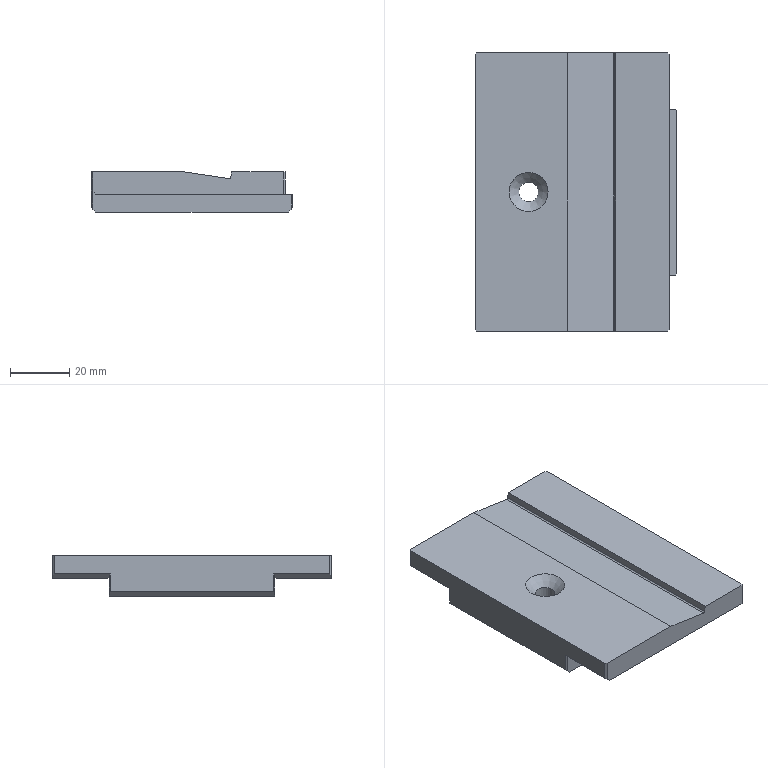NC program | NX | posted with a generic post | part box 68 x 94 x 13.65 mm
Lines 1 to 1097 of 5620:
N10 G17 G21 G94 G90
(一刀光面 , TOOL : D50面刀)
N12 T01 M6
N14 G54
N16 G17 G0 G90 X78.5 Y-22.5 B0. C0. S3500 M3
N18 G43 Z30. H1
N20 Z3.
N22 G94 G1 Z0. F800.
N24 X73.5
N26 X-73.5
N28 X-78.5
N30 Z3.
N32 G0 Z30.
N34 X78.5 Y15.
N36 Z3.
N38 G1 Z0.
N40 X73.5
N42 X-73.5
N44 X-78.5
N46 Z3.
N48 G0 Z30.
N50 M5
(ADAPTIVE_MILLING , TOOL : D12开粗)
N52 T02 M6
N54 G54
N56 G17 G0 G90 X0.814 Y-47.076 B0. C0. S6500 M3
N58 G43 Z30. H2
N60 Z-13.
N62 G94 G1 Y-46.926 Z-13.937 F2500.
N64 Y-46.776 Z-14.308
N66 Y-46.626 Z-14.58
N68 X0.815 Y-46.476 Z-14.8
N70 Y-46.326 Z-14.984
N72 Y-46.176 Z-15.142
N74 X0.816 Y-46.026 Z-15.28
N76 Y-45.876 Z-15.4
N78 Y-45.726 Z-15.505
N80 X0.817 Y-45.576 Z-15.598
N82 Y-45.426 Z-15.679
N84 Y-45.276 Z-15.75
N86 X0.818 Y-45.126 Z-15.81
N88 Y-44.976 Z-15.862
N90 Y-44.826 Z-15.905
N92 X0.819 Y-44.676 Z-15.939
N94 Y-44.526 Z-15.966
N96 Y-44.376 Z-15.985
N98 X0.82 Y-44.226 Z-15.996
N100 Y-44.076 Z-16.
N102 X0.824 Y-42.206
N104 G3 X0.012 Y-41.059 R1.212
N106 X-2.89 Y-40.578 R11.249
N108 X-11.498 Y-40.406 R147.652
N110 G1 X-18.236 Y-40.4
N112 X-45.986 Y-40.399
N114 G2 X-48.611 Y-39.755 R6.142
N116 G1 X-48.855 Y-39.681
N118 X-49.918 Y-39.113
N120 G2 X-52.114 Y-36.915 R10.677
N122 X-52.788 Y-35.571 R9.839
N124 X-53.72 Y-30.116 R21.533
N126 X-53.893 Y-21.344 R159.693
N128 G1 X-53.899 Y-14.594
N130 X-53.898 Y32.484
N132 G2 X-51.638 Y37.222 R6.591
N134 X-46.864 Y39.623 R10.72
N136 X-40.988 Y40.3 R29.653
N138 X-27.714 Y40.399 R443.721
N140 G1 X46.082 Y40.397
N142 G2 X50.795 Y38.079 R6.624
N144 X53.148 Y33.282 R10.797
N146 X53.803 Y27.403 R30.317
N148 X53.899 Y13.453 R504.778
N150 G1 X53.898 Y-32.465
N152 G2 X52.294 Y-36.579 R6.493
N154 G1 X52.113 Y-36.918
N156 G2 X49.915 Y-39.114 R10.677
N158 G1 X48.852 Y-39.682
N160 X47.551 Y-40.06
N162 G2 X39.986 Y-40.38 R73.937
N164 G1 X30.536 Y-40.399
N166 X-42.041 Y-40.394
N168 G3 X-43.223 Y-40.15 R35.364
N170 G1 X-46.501
N172 X-47.701 Y-40.031
N174 X-48.855 Y-39.681
N176 X-49.918 Y-39.113
N178 G2 X-52.114 Y-36.915 R10.677
N180 G1 X-52.682 Y-35.852
N182 X-53.032 Y-34.698
N184 X-53.15 Y-33.499
N186 G3 X-53.259 Y-25.386 R401.161
N188 G1 X-53.298 Y-13.836
N190 Y29.859
N192 G2 X-52.591 Y33.461 R9.973
N194 X-48.087 Y37.818 R9.638
N196 X-42.325 Y39.395 R17.668
N198 X-34.538 Y39.77 R72.985
N200 G1 X-29.459 Y39.811
N202 X-28.698 Y40.032
N204 X-27.499 Y40.15
N206 X27.501
N208 G3 X34.729 Y39.821 R67.085
N210 G1 X43.91 Y39.783
N212 G2 X50.284 Y36.226 R8.601
N214 X52.114 Y34.315 R10.653
N216 G1 X52.682 Y33.252
N218 X53.032 Y32.098
N220 G2 X53.159 Y29.701 R16.371
N222 X53.298 Y11.488 R714.314
N224 G1 X53.297 Y-30.033
N226 G2 X53.15 Y-31.551 R14.853
N228 G1 Y-33.501
N230 X53.031 Y-34.701
N232 X52.681 Y-35.855
N234 X52.292 Y-36.582
N236 G3 X54.371 Y-37.779 R1.2
N238 G1 X54.7 Y-37.246
N240 X55.951 Y-35.222 Z-15.9
N242 X56.104 Y-34.976 F15000.
N244 X56.246 Y-34.723
N246 G3 X56.348 Y-34.241 R1.247
N248 G1 X56.462 Y26.838
N250 X56.449 Y26.999
N252 X56.418 Y27.159
N254 X56.128 Y28.213
N256 X55.496 Y30.506 Z-16. F2500.
N258 G3 X53.15 Y30.149 R1.2
N260 G1 Y-33.501
N262 X53.031 Y-34.701
N264 X52.681 Y-35.855
N266 X52.113 Y-36.918
N268 G2 X49.915 Y-39.114 R10.677
N270 G1 X48.852 Y-39.682
N272 X47.698 Y-40.032
N274 X46.5 Y-40.15
N276 X-46.501
N278 X-47.701 Y-40.031
N280 X-48.855 Y-39.681
N282 X-49.918 Y-39.113
N284 G2 X-52.114 Y-36.915 R10.677
N286 G1 X-52.682 Y-35.852
N288 X-53.032 Y-34.698
N290 X-53.15 Y-33.499
N292 Y30.901
N294 X-53.031 Y32.101
N296 X-52.681 Y33.255
N298 X-52.113 Y34.318
N300 G2 X-49.915 Y36.514 R10.677
N302 G1 X-48.713 Y37.139
N304 G2 X-38.58 Y39.001 R35.913
N306 X-31.101 Y39.2 R262.378
N308 G3 X-30.519 Y39.326 R1.742
N310 G2 X-29.35 Y39.835 R4.049
N312 G3 X-29.125 Y42.27 R1.32
N314 X-30.028 Y42.389 Z-15.961 R1.4
N316 G1 X-31.464 Y42.187 Z-15.9
N318 X-43.233 Y40.526 F15000.
N320 X-45.589 Y40.193 Z-16. F2500.
N322 X-49.419 Y39.653
N324 G3 X-48.852 Y37.082 R-1.32
N326 G1 X-47.698 Y37.432
N328 G3 X-41.358 Y38.14 R635.972
N330 G2 X-32.831 Y38.561 R125.688
N332 G3 X-31.416 Y38.765 R4.842
N334 X-30.915 Y39.114 R2.568
N336 G1 X-30.519 Y39.326
N338 G3 X-30.15 Y41.363 R1.32
N340 X-31.39 Y41.792 Z-15.942 R1.359
N342 G1 X-32.393 Y41.686 Z-15.9
N344 X-43.396 Y40.525 F15000.
N346 X-45.762 Y40.275 Z-16. F2500.
N348 X-46.287 Y40.223
N350 X-46.809 Y40.153
N352 G3 X-46.499 Y37.55 R1.32
N354 X-38.557 Y37.753 R103.824
N356 X-33.424 Y37.981 R179.629
N358 X-31.964 Y38.284 R4.532
N360 X-31.123 Y38.944 R9.125
N362 X-30.883 Y40.727 R1.32
N364 X-32.198 Y41.267 Z-15.937 R1.355
N366 G1 X-33.074 Y41.182 Z-15.9
N368 X-39.775 Y40.525 F15000.
N370 X-42.142 Y40.293 Z-16. F2500.
N372 X-43.253 Y40.184
N374 G3 X-43.124 Y37.55 R1.32
N376 G1 X-33.996 Y37.558
N378 G3 X-32.424 Y37.854 R4.372
N380 X-31.79 Y38.397 R3.138
N382 X-33.061 Y40.664 R1.32
N384 G1 X-34.633 Y40.117
N386 G3 X-34.199 Y37.55 R1.32
N388 X-32.924 Y37.593 R6.49
N390 X-32.159 Y38.038 R1.604
N392 X-31.814 Y38.861 R1.203
N394 G1 X-31.801 Y39.652
N396 X-31.762 Y42.031 Z-15.9
N398 G2 X-30.774 Y43.208 R1.2 F15000.
N400 G1 X-29.753 Y43.392
N402 X-28.73 Y43.564
N404 G2 X-26.371 Y43.734 R17.038
N406 G1 X24.917 Y43.816
N408 G2 X25.87 Y43.347 R1.201
N410 G1 X26.035 Y43.133
N412 X27.484 Y41.247 Z-16. F2500.
N414 X27.834 Y40.787
N416 X28.196 Y40.336
N418 G3 X28.701 Y40.031 R1.217
N420 X32.386 Y39.4 R14.318
N422 X41.453 Y39.203 R159.798
N424 G2 X46.995 Y37.575 R10.592
N426 G3 X47.701 Y37.431 R2.022
N428 G1 X48.855 Y37.081
N430 X49.918 Y36.513
N432 X50.382 Y36.132
N434 G3 X52.103 Y37.78 R1.2
N436 G1 X50.521 Y39.557 Z-15.9
N438 X49.885 Y40.268 F15000.
N440 G3 X49.17 Y40.656 R1.205
N442 G1 X32.659 Y43.147
N444 G3 X32.082 Y43.093 R1.219
N446 G1 X30.6 Y42.573
N448 X29.909 Y42.333 Z-15.931 F2500.
N450 X29.222 Y42.083 Z-15.962
N452 G3 X28.591 Y41.452 Z-16. R1.2
N454 X29.347 Y39.835 R1.2
N456 G2 X30.562 Y39.404 R18.042
N458 G3 X34.903 Y38.786 R19.773
N460 X40.407 Y38.596 R594.107
N462 G2 X44.603 Y37.696 R16.331
N464 G3 X45.182 Y37.55 R5.874
N466 G2 X47.396 Y37.461 R14.116
N468 G3 X47.683 Y40.086 R1.32
N470 G1 X46.405 Y40.239
N472 X44.044 Y40.522 Z-15.9
N474 X31.872 Y41.98 F15000.
N476 X30.615 Y42.125 Z-15.953 F2500.
N478 G3 X29.607 Y41.74 Z-16. R1.319
N480 X29.921 Y39.646 R1.32
N482 X33.274 Y38.529 R8.778
N484 X38.564 Y38.088 R53.298
N486 G2 X42.311 Y37.55 R28.728
N488 G1 X45.236
N490 G3 X45.382 Y40.182 R1.32
N492 G1 X44.683 Y40.259
N494 X42.318 Y40.522 Z-15.9
N496 X32.542 Y41.608 F15000.
N498 X31.903 Y41.683 Z-15.927 F2500.
N500 X31.261 Y41.741 Z-15.954
N502 G3 X30.294 Y41.308 Z-16. R1.334
N504 X30.648 Y39.257 R1.32
N506 X32.25 Y38.473 R8.689
N508 X36.232 Y37.737 R18.874
N510 G1 X38.011 Y37.55
N512 X42.361
N514 G3 X42.517 Y40.181 R1.32
N516 G1 X42.014 Y40.241
N518 X39.651 Y40.522 Z-15.9
N520 X32.922 Y41.323 F15000.
N522 X31.827 Y41.448 Z-15.946 F2500.
N524 G3 X30.711 Y40.94 Z-16. R1.319
N526 X30.918 Y39.113 R1.32
N528 X33.301 Y37.863 R5.718
N530 X34.636 Y37.55 R19.176
N532 G1 X38.086
N534 G3 X38.334 Y40.166 R1.32
N536 G1 X35.982 Y40.521 Z-15.9
N538 X33.433 Y40.904 F15000.
N540 X32.331 Y41.065 Z-15.947 F2500.
N542 G3 X31.208 Y40.6 Z-16. R1.319
N544 X31.382 Y38.732 R1.32
N546 X33.394 Y37.568 R5.026
N548 X34.668 Y37.55 R53.565
N550 X34.95 Y40.16 R1.32
N552 G1 X33.064 Y40.572
N554 G3 X31.849 Y38.348 R1.32
N556 X32.694 Y37.663 R3.182
N558 X33.563 Y37.55 R2.269
N560 X33.826 Y40.164 R1.32
N562 G1 X33.508 Y40.23
N564 X33.187 Y40.281
N566 G3 X32.168 Y38.03 R1.32
N568 X32.615 Y37.705 R2.445
N570 X34.332 Y39.066 R1.212
N572 G1 X33.995 Y40.523
N574 X33.961 Y40.67 Z-15.996
N576 X33.927 Y40.816 Z-15.985
N578 X33.893 Y40.962 Z-15.966
N580 X33.859 Y41.108 Z-15.939
N582 X33.826 Y41.254 Z-15.905
N584 X33.792 Y41.4 Z-15.862
N586 X33.758 Y41.546 Z-15.81
N588 X33.724 Y41.693 Z-15.75
N590 X33.69 Y41.839 Z-15.679
N592 X33.656 Y41.985 Z-15.598
N594 X33.623 Y42.131 Z-15.505
N596 X33.589 Y42.277 Z-15.4
N598 X33.555 Y42.423 Z-15.28
N600 X33.521 Y42.569 Z-15.142
N602 X33.487 Y42.716 Z-14.984
N604 X33.453 Y42.862 Z-14.8
N606 X33.42 Y43.008 Z-14.58
N608 X33.386 Y43.154 Z-14.308
N610 X33.352 Y43.3 Z-13.937
N612 X33.318 Y43.446 Z-13.
N614 G0 Z30.
N616 X-34.093 Y43.523
N618 Z-4.5
N620 G1 X-34.096 Y43.373 Z-5.437
N622 X-34.1 Y43.223 Z-5.808
N624 X-34.104 Y43.073 Z-6.08
N626 X-34.107 Y42.923 Z-6.3
N628 X-34.111 Y42.773 Z-6.484
N630 X-34.115 Y42.623 Z-6.642
N632 X-34.118 Y42.473 Z-6.78
N634 X-34.122 Y42.323 Z-6.9
N636 X-34.126 Y42.173 Z-7.005
N638 X-34.129 Y42.023 Z-7.098
N640 X-34.133 Y41.873 Z-7.179
N642 X-34.137 Y41.723 Z-7.25
N644 X-34.14 Y41.573 Z-7.31
N646 X-34.144 Y41.423 Z-7.362
N648 X-34.148 Y41.273 Z-7.405
N650 X-34.151 Y41.123 Z-7.439
N652 X-34.155 Y40.973 Z-7.466
N654 X-34.159 Y40.823 Z-7.485
N656 X-34.162 Y40.673 Z-7.496
N658 X-34.166 Y40.523 Z-7.5
N660 X-34.207 Y38.861
N662 G3 X-32.677 Y37.662 R1.212
N664 X-31.366 Y38.234 R46.348
N666 G2 X-26.093 Y39.31 R18.668
N668 X-17.848 Y39.529 R115.828
N670 G1 X-9.898 Y39.538
N672 X26.476 Y39.533
N674 G2 X30.128 Y38.198 R14.941
N676 G3 X31.607 Y37.572 R10.585
N678 X32.969 Y37.55 R11.475
N680 X34.162 Y38.883 R1.2
N682 X33.567 Y39.796 Z-7.453 R1.255
N684 G1 X32.546 Y40.516 Z-7.4
N686 X31.31 Y41.387 F15000.
N688 G3 X30.628 Y41.606 R1.208
N690 G1 X-31.7 Y42.074
N692 G3 X-32.755 Y41.462 R1.201
N694 G1 X-33.274 Y40.54
N696 X-33.635 Y39.904 Z-7.431 F2500.
N698 X-33.986 Y39.263 Z-7.462
N700 G3 X-34.043 Y38.372 Z-7.5 R1.2
N702 X-32.912 Y37.55 R1.2
N704 X-29.647 Y38.155 R77.338
N706 G2 X-21.135 Y38.864 R56.46
N708 X-7.186 Y38.938 R788.437
N710 G1 X25.801 Y38.932
N712 G2 X29.491 Y37.708 R34.361
N714 G3 X30.096 Y37.55 R3.366
N716 G1 X31.821
N718 G3 X33.014 Y38.879 R1.2
N720 X32.421 Y39.795 Z-7.453 R1.255
N722 G1 X31.402 Y40.516 Z-7.4
N724 X30.172 Y41.386 F15000.
N726 G3 X29.479 Y41.606 R1.208
N728 G1 X-30.57
N730 G3 X-31.263 Y41.386 R1.208
N732 G1 X-32.467 Y40.534
N734 X-33.071 Y40.11 Z-7.431 F2500.
N736 X-33.668 Y39.678 Z-7.462
N738 G3 X-34.101 Y38.91 Z-7.5 R1.2
N740 X-32.912 Y37.55 R1.2
N742 X-29.528 Y37.694 R26.636
N744 G2 X-16.282 Y38.312 R132.735
N746 G1 X-5.032 Y38.337
N748 X24.151 Y38.332
N750 G2 X27.654 Y37.561 R34.199
N752 G1 X30.15 Y37.55
N754 G3 X31.343 Y38.879 R1.2
N756 X30.75 Y39.795 Z-7.453 R1.255
N758 G1 X29.73 Y40.516 Z-7.4
N760 X28.501 Y41.386 F15000.
N762 G3 X27.808 Y41.606 R1.208
N764 G1 X-29.22
N766 G3 X-29.913 Y41.386 R1.208
N768 G1 X-31.117 Y40.534
N770 X-31.721 Y40.11 Z-7.431 F2500.
N772 X-32.318 Y39.678 Z-7.462
N774 G3 X-32.751 Y38.91 Z-7.5 R1.2
N776 X-31.562 Y37.55 R1.2
N778 X-18.981 Y37.672 R367.675
N780 G2 X-3.531 Y37.737 R890.928
N782 G1 X21.827 Y37.731
N784 G2 X23.908 Y37.55 R42.866
N786 G1 X27.808
N788 G3 X28.191 Y39.887 R1.2
N790 G1 X25.898 Y40.52 Z-7.4
N792 X24.815 Y40.818 F15000.
N794 X24.656 Y40.849
N796 X24.496 Y40.861
N798 X-21.575 Y40.862
N800 X-21.736 Y40.849
N802 X-21.894 Y40.819
N804 X-22.952 Y40.527
N806 X-25.246 Y39.895 Z-7.5 F2500.
N808 G3 X-24.887 Y37.55 R1.2
N810 G1 X23.938
N812 G3 X25.138 Y38.588 R1.212
N814 G1 X25.417 Y40.523
N816 X25.439 Y40.672 Z-7.496
N818 X25.46 Y40.82 Z-7.485
N820 X25.482 Y40.969 Z-7.466
N822 X25.503 Y41.117 Z-7.439
N824 X25.525 Y41.266 Z-7.405
N826 X25.546 Y41.414 Z-7.362
N828 X25.568 Y41.563 Z-7.31
N830 X25.589 Y41.711 Z-7.25
N832 X25.611 Y41.86 Z-7.179
N834 X25.632 Y42.008 Z-7.098
N836 X25.654 Y42.156 Z-7.005
N838 X25.675 Y42.305 Z-6.9
N840 X25.697 Y42.453 Z-6.78
N842 X25.718 Y42.602 Z-6.642
N844 X25.739 Y42.75 Z-6.484
N846 X25.761 Y42.899 Z-6.3
N848 X25.782 Y43.047 Z-6.08
N850 X25.804 Y43.196 Z-5.808
N852 X25.825 Y43.344 Z-5.437
N854 X25.847 Y43.493 Z-4.5
N856 G0 Z30.
N858 X-59.083 Y5.759
N860 Z1.5
N862 G1 X-58.935 Y5.784 Z0.563
N864 X-58.787 Y5.808 Z0.192
N866 X-58.639 Y5.833 Z-0.08
N868 X-58.491 Y5.857 Z-0.3
N870 X-58.343 Y5.882 Z-0.484
N872 X-58.195 Y5.906 Z-0.642
N874 X-58.047 Y5.931 Z-0.78
N876 X-57.899 Y5.955 Z-0.9
N878 X-57.751 Y5.98 Z-1.005
N880 X-57.603 Y6.004 Z-1.098
N882 X-57.455 Y6.028 Z-1.179
N884 X-57.307 Y6.053 Z-1.25
N886 X-57.159 Y6.077 Z-1.31
N888 X-57.011 Y6.102 Z-1.362
N890 X-56.863 Y6.126 Z-1.405
N892 X-56.715 Y6.151 Z-1.439
N894 X-56.567 Y6.175 Z-1.466
N896 X-56.419 Y6.2 Z-1.485
N898 X-56.271 Y6.224 Z-1.496
N900 X-56.123 Y6.249 Z-1.5
N902 X-54.112 Y6.581
N904 G3 X-53.101 Y7.685 R1.212
N906 G2 X-52.86 Y9.444 R9.582
N908 G3 X-52.717 Y10.845 R6.707
N910 G1 X-53.04 Y11.994
N912 X-53.062 Y12.218
N914 G3 X-55.695 Y12.045 R1.32
N916 G1 X-55.586 Y9.045
N918 G3 X-52.982 Y8.792 R1.32
N920 X-52.645 Y10.429 R11.274
N922 X-52.747 Y10.995 R5.595
N924 X-53.935 Y11.865 R1.212
N926 G1 X-56.011 Y11.821
N928 X-56.161 Y11.818 Z-1.496
N930 X-56.311 Y11.815 Z-1.485
N932 X-56.461 Y11.811 Z-1.466
N934 X-56.611 Y11.808 Z-1.439
N936 X-56.761 Y11.805 Z-1.405
N938 X-56.911 Y11.802 Z-1.362
N940 X-57.061 Y11.799 Z-1.31
N942 X-57.211 Y11.796 Z-1.25
N944 X-57.361 Y11.792 Z-1.179
N946 X-57.511 Y11.789 Z-1.098
N948 X-57.66 Y11.786 Z-1.005
N950 X-57.81 Y11.783 Z-0.9
N952 X-57.96 Y11.78 Z-0.78
N954 X-58.11 Y11.776 Z-0.642
N956 X-58.26 Y11.773 Z-0.484
N958 X-58.41 Y11.77 Z-0.3
N960 X-58.56 Y11.767 Z-0.08
N962 X-58.71 Y11.764 Z0.192
N964 X-58.86 Y11.761 Z0.563
N966 X-59.01 Y11.757 Z1.5
N968 G0 Z30.
N970 X-59.108 Y2.742
N972 Z2.
N974 G1 X-58.959 Y2.757 Z1.063
N976 X-58.809 Y2.772 Z0.692
N978 X-58.66 Y2.787 Z0.42
N980 X-58.511 Y2.802 Z0.2
N982 X-58.362 Y2.817 Z0.016
N984 X-58.212 Y2.832 Z-0.142
N986 X-58.063 Y2.847 Z-0.28
N988 X-57.914 Y2.862 Z-0.4
N990 X-57.765 Y2.877 Z-0.505
N992 X-57.615 Y2.892 Z-0.598
N994 X-57.466 Y2.907 Z-0.679
N996 X-57.317 Y2.922 Z-0.75
N998 X-57.168 Y2.937 Z-0.81
N1000 X-57.018 Y2.952 Z-0.862
N1002 X-56.869 Y2.967 Z-0.905
N1004 X-56.72 Y2.982 Z-0.939
N1006 X-56.571 Y2.997 Z-0.966
N1008 X-56.421 Y3.012 Z-0.985
N1010 X-56.272 Y3.027 Z-0.996
N1012 X-56.123 Y3.042 Z-1.
N1014 X-54.189 Y3.237
N1016 G3 X-53.103 Y4.338 R1.212
N1018 G2 X-52.656 Y7.193 R22.
N1020 G3 X-52.303 Y9.906 R12.298
N1022 X-52.422 Y10.338 R4.094
N1024 X-54.046 Y10.957 R1.32
N1026 X-54.908 Y9.821 Z-0.937 R1.355
N1028 G1 X-55.047 Y8.957 Z-0.9
N1030 X-55.109 Y8.575 F15000.
N1032 X-55.399 Y6.746 Z-0.978 F2500.
N1034 G3 X-55.351 Y6.225 Z-1. R1.34
N1036 X-52.848 Y6.16 R1.32
N1038 X-52.087 Y8.596 R14.
N1040 X-52.129 Y9.846 R2.391
N1042 G2 X-52.727 Y11.041 R6.81
N1044 G3 X-54.995 Y11.335 R1.32
N1046 X-55.241 Y10.26 Z-0.952 R1.378
N1048 G1 X-55.088 Y9.027 Z-0.9
N1050 X-55.048 Y8.701 F15000.
N1052 X-54.907 Y7.616 Z-0.946 F2500.
N1054 G3 X-54.139 Y6.652 Z-1. R1.319
N1056 X-52.469 Y7.205 R1.32
N1058 X-51.857 Y9.222 R3.346
N1060 X-52.195 Y9.981 R1.76
N1062 X-54.635 Y9.332 R1.32
N1064 G1 X-54.671 Y8.367
N1066 G3 X-52.207 Y7.66 R1.32
N1068 X-51.733 Y8.851 R2.605
N1070 X-52.018 Y9.697 R1.658
N1072 X-53.971 Y7.975 R-1.32
N1074 X-52.742 Y7.635 R1.374
N1076 X-51.781 Y8.53 R1.321
N1078 G1 X-51.757 Y8.605
N1080 X-51.742 Y8.754
N1082 G3 X-54.166 Y9.145 R1.232
N1084 X-51.808 Y8.44 R-1.23
N1086 X-53.71 Y9.755 R1.212
N1088 G1 X-55.018 Y8.738
N1090 X-55.137 Y8.646 Z-0.996
N1092 X-55.255 Y8.553 Z-0.985
N1094 X-55.373 Y8.461 Z-0.966
N1096 X-55.492 Y8.369 Z-0.939
N1098 X-55.61 Y8.277 Z-0.905
N1100 X-55.728 Y8.185 Z-0.862
N1102 X-55.847 Y8.093 Z-0.81
N1104 X-55.965 Y8.001 Z-0.75
N1106 X-56.084 Y7.909 Z-0.679
N1108 X-56.202 Y7.817 Z-0.598
N1110 X-56.32 Y7.725 Z-0.505
N1112 X-56.439 Y7.632 Z-0.4
N1114 X-56.557 Y7.54 Z-0.28
N1116 X-56.676 Y7.448 Z-0.142
N1118 X-56.794 Y7.356 Z0.016
N1120 X-56.912 Y7.264 Z0.2
N1122 X-57.031 Y7.172 Z0.42
N1124 X-57.149 Y7.08 Z0.692
N1126 X-57.268 Y6.988 Z1.063
N1128 X-57.386 Y6.896 Z2.
N1130 G0 Z30.
N1132 X-59.111 Y0.175
N1134 Z2.5
N1136 G1 X-58.962 Y0.161 Z1.563
N1138 X-58.812 Y0.148 Z1.192
N1140 X-58.663 Y0.135 Z0.92
N1142 X-58.513 Y0.121 Z0.7
N1144 X-58.364 Y0.108 Z0.516
N1146 X-58.215 Y0.095 Z0.358
N1148 X-58.065 Y0.081 Z0.22
N1150 X-57.916 Y0.068 Z0.1
N1152 X-57.766 Y0.055 Z-0.005
N1154 X-57.617 Y0.041 Z-0.098
N1156 X-57.468 Y0.028 Z-0.179
N1158 X-57.318 Y0.015 Z-0.25
N1160 X-57.169 Y0.001 Z-0.31
N1162 X-57.019 Y-0.012 Z-0.362
N1164 X-56.87 Y-0.025 Z-0.405
N1166 X-56.721 Y-0.039 Z-0.439
N1168 X-56.571 Y-0.052 Z-0.466
N1170 X-56.422 Y-0.065 Z-0.485
N1172 X-56.272 Y-0.079 Z-0.496
N1174 X-56.123 Y-0.092 Z-0.5
N1176 X-54.428 Y-0.243
N1178 G3 X-53.113 Y0.864 R1.212
N1180 G2 X-51.99 Y5.996 R18.609
N1182 G3 X-51.467 Y8.295 R7.898
N1184 X-51.763 Y9.463 R2.025
N1186 G1 X-52.138 Y9.927
N1188 X-52.592 Y10.79
N1190 G3 X-54.37 Y11.346 R1.32
N1192 X-55.084 Y10.128 Z-0.438 R1.356
N1194 G1 X-55.128 Y9.237 Z-0.4
N1196 X-55.354 Y4.652 F15000.
N1198 X-55.419 Y3.211 Z-0.461 F2500.
N1200 G3 X-55.09 Y2.356 Z-0.5 R1.32
N1202 X-52.859 Y2.787 R1.32
N1204 G2 X-52.068 Y4.672 R11.566
N1206 G3 X-51.193 Y7.786 R8.801
N1208 X-51.447 Y9.072 R2.096
N1210 G1 X-51.777 Y9.481
N1212 G3 X-53.275 Y9.885 R1.32
N1214 X-54.122 Y8.79 Z-0.439 R1.359
N1216 G1 X-54.298 Y7.882 Z-0.4
N1218 X-54.66 Y6.017 F15000.
N1220 X-54.912 Y4.693 Z-0.457 F2500.
N1222 G3 X-54.658 Y3.722 Z-0.5 R1.32
N1224 X-52.459 Y3.867 R1.32
N1226 G1 X-51.541 Y5.423
N1228 G3 X-50.983 Y8.289 R4.803
N1230 X-51.326 Y8.945 R1.429
N1232 X-52.639 Y9.228 R1.321
N1234 X-53.515 Y8.265 Z-0.443 R1.364
N1236 G1 X-53.823 Y7.293 Z-0.4
N1238 X-53.89 Y7.079 F15000.
N1240 X-54.079 Y6.487 Z-0.426 F2500.
N1242 X-54.259 Y5.893 Z-0.452
N1244 G3 X-54.053 Y4.812 Z-0.5 R1.319
N1246 X-51.963 Y4.738 R1.32
N1248 X-50.724 Y7.57 R4.383
N1250 X-51.389 Y9. R1.56
N1252 G1 X-51.483 Y9.117
N1254 G3 X-53.167 Y9.433 R1.32
N1256 X-53.83 Y8.173 Z-0.437 R1.355
N1258 G1 X-53.827 Y7.296 Z-0.4
N1260 X-53.826 Y7.161 F15000.
N1262 X-53.816 Y6.067 Z-0.446 F2500.
N1264 G3 X-53.168 Y5.018 Z-0.5 R1.319
N1266 X-51.485 Y5.316 R1.32
N1268 X-50.586 Y7.954 R3.153
N1270 X-51.199 Y8.84 R1.436
N1272 X-53.364 Y7.918 R1.32
N1274 G1 X-53.449 Y6.663
N1276 G3 X-51.276 Y5.569 R1.32
N1278 X-50.473 Y8.014 R2.376
N1280 X-50.976 Y8.653 R1.462
N1282 X-53.13 Y7.836 R1.32
N1284 G1 X-53.267 Y6.913
N1286 G3 X-51.105 Y5.715 R1.32
N1288 X-50.313 Y7.835 R2.086
N1290 X-50.835 Y8.535 R1.425
N1292 X-52.999 Y7.631 R1.32
N1294 G1 X-53.033 Y7.24
N1296 X-53.051 Y6.848
N1298 G3 X-50.876 Y5.91 R1.32
N1300 X-50.202 Y7.757 R1.758
N1302 X-50.708 Y8.428 R1.427
N1304 X-50.854 Y5.944 R-1.553
N1306 X-50.069 Y7.51 R1.604
N1308 X-50.578 Y8.32 R1.359
N1310 X-52.583 Y6.54 R1.356
N1312 X-50.452 Y6.277 R1.391
N1314 X-50.345 Y8.099 R1.248
N1316 X-51.834 Y8.346 R1.212
N1318 G1 X-53.8 Y7.253
N1320 X-53.931 Y7.18 Z-0.496
N1322 X-54.062 Y7.107 Z-0.485
N1324 X-54.193 Y7.034 Z-0.466
N1326 X-54.324 Y6.961 Z-0.439
N1328 X-54.456 Y6.888 Z-0.405
N1330 X-54.587 Y6.815 Z-0.362
N1332 X-54.718 Y6.742 Z-0.31
N1334 X-54.849 Y6.669 Z-0.25
N1336 X-54.98 Y6.597 Z-0.179
N1338 X-55.111 Y6.524 Z-0.098
N1340 X-55.242 Y6.451 Z-0.005
N1342 X-55.373 Y6.378 Z0.1
N1344 X-55.504 Y6.305 Z0.22
N1346 X-55.635 Y6.232 Z0.358
N1348 X-55.767 Y6.159 Z0.516
N1350 X-55.898 Y6.086 Z0.7
N1352 X-56.029 Y6.013 Z0.92
N1354 X-56.16 Y5.94 Z1.192
N1356 X-56.291 Y5.868 Z1.563
N1358 X-56.422 Y5.795 Z2.5
N1360 G0 Z30.
N1362 X59.079 Y14.124
N1364 Z1.5
N1366 G1 X58.931 Y14.098 Z0.563
N1368 X58.784 Y14.072 Z0.192
N1370 X58.636 Y14.047 Z-0.08
N1372 X58.488 Y14.021 Z-0.3
N1374 X58.34 Y13.995 Z-0.484
N1376 X58.192 Y13.969 Z-0.642
N1378 X58.045 Y13.944 Z-0.78
N1380 X57.897 Y13.918 Z-0.9
N1382 X57.749 Y13.892 Z-1.005
N1384 X57.601 Y13.867 Z-1.098
N1386 X57.453 Y13.841 Z-1.179
N1388 X57.306 Y13.815 Z-1.25
N1390 X57.158 Y13.79 Z-1.31
N1392 X57.01 Y13.764 Z-1.362
N1394 X56.862 Y13.738 Z-1.405
N1396 X56.715 Y13.713 Z-1.439
N1398 X56.567 Y13.687 Z-1.466
N1400 X56.419 Y13.661 Z-1.485
N1402 X56.271 Y13.636 Z-1.496
N1404 X56.123 Y13.61 Z-1.5
N1406 X54.054 Y13.25
N1408 G3 X53.055 Y12.172 R1.212
N1410 X52.746 Y9.894 R27.542
N1412 X52.941 Y9.049 R4.487
N1414 G2 X53.111 Y7.824 R13.191
N1416 G3 X54.495 Y6.571 R1.32
N1418 X55.748 Y7.943 R1.32
N1420 G1 X55.6 Y11.589
N1422 G3 X53.015 Y11.91 R1.32
N1424 X52.634 Y10.402 R7.546
N1426 X52.774 Y9.664 R3.953
N1428 X53.977 Y8.771 R1.212
N1430 G1 X55.987 Y8.827
N1432 X56.137 Y8.831 Z-1.496
N1434 X56.287 Y8.835 Z-1.485
N1436 X56.437 Y8.84 Z-1.466
N1438 X56.587 Y8.844 Z-1.439
N1440 X56.737 Y8.848 Z-1.405
N1442 X56.887 Y8.852 Z-1.362
N1444 X57.037 Y8.856 Z-1.31
N1446 X57.187 Y8.86 Z-1.25
N1448 X57.337 Y8.865 Z-1.179
N1450 X57.487 Y8.869 Z-1.098
N1452 X57.637 Y8.873 Z-1.005
N1454 X57.787 Y8.877 Z-0.9
N1456 X57.936 Y8.881 Z-0.78
N1458 X58.086 Y8.885 Z-0.642
N1460 X58.236 Y8.89 Z-0.484
N1462 X58.386 Y8.894 Z-0.3
N1464 X58.536 Y8.898 Z-0.08
N1466 X58.686 Y8.902 Z0.192
N1468 X58.836 Y8.906 Z0.563
N1470 X58.986 Y8.91 Z1.5
N1472 G0 Z30.
N1474 X58.98 Y11.587
N1476 Z2.
N1478 G1 X58.83 Y11.59 Z1.063
N1480 X58.68 Y11.593 Z0.692
N1482 X58.53 Y11.596 Z0.42
N1484 X58.38 Y11.599 Z0.2
N1486 X58.23 Y11.603 Z0.016
N1488 X58.08 Y11.606 Z-0.142
N1490 X57.93 Y11.609 Z-0.28
N1492 X57.78 Y11.612 Z-0.4
N1494 X57.63 Y11.615 Z-0.505
N1496 X57.48 Y11.618 Z-0.598
N1498 X57.33 Y11.621 Z-0.679
N1500 X57.18 Y11.624 Z-0.75
N1502 X57.03 Y11.627 Z-0.81
N1504 X56.88 Y11.631 Z-0.862
N1506 X56.73 Y11.634 Z-0.905
N1508 X56.58 Y11.637 Z-0.939
N1510 X56.43 Y11.64 Z-0.966
N1512 X56.28 Y11.643 Z-0.985
N1514 X56.13 Y11.646 Z-0.996
N1516 X55.98 Y11.649 Z-1.
N1518 X53.833 Y11.694
N1520 G3 X52.692 Y10.954 R1.212
N1522 X52.553 Y9.773 R2.798
N1524 G1 X52.563 Y7.018
N1526 G3 X52.847 Y6.17 R7.827
N1528 G2 X53.116 Y4.19 R12.907
N1530 G3 X55.745 Y4.431 R-1.32
N1532 G1 X55.649 Y5.416
N1534 X55.42 Y7.784 Z-0.9
N1536 X55.264 Y9.385 F15000.
N1538 X55.15 Y10.511 Z-0.948 F2500.
N1540 G3 X54.443 Y11.481 Z-1. R1.319
N1542 X52.633 Y10.816 R1.32
N1544 X52.188 Y7.86 R7.548
N1546 X52.47 Y7.204 R1.829
N1548 G1 X52.624 Y6.781
N1550 G3 X54.74 Y6.247 R1.32
N1552 X55.179 Y7.392 Z-0.947 R1.365
N1554 G1 X55.14 Y8.497 Z-0.9
N1556 X55.119 Y9.064 F15000.
N1558 X55.073 Y10.223 Z-0.949 F2500.
N1560 G3 X54.451 Y11.22 Z-1. R1.319
N1562 X52.546 Y10.609 R1.32
N1564 X51.943 Y8.427 R5.287
N1566 X52.308 Y7.483 R1.909
N1568 X54.765 Y8.04 R1.32
N1570 G1 X54.89 Y9.587
N1572 G3 X52.455 Y10.394 R1.32
N1574 X51.792 Y8.691 R3.327
N1576 X52.105 Y7.832 R1.654
N1578 X54.567 Y8.478 R1.32
N1580 G1 X54.574 Y8.909
N1582 X54.566 Y9.339
N1584 G3 X52.137 Y9.885 R1.32
N1586 X51.73 Y8.846 R1.917
N1588 X51.921 Y8.159 R1.633
N1590 X53.265 Y7.519 R1.212
N1592 G1 X55.352 Y7.978
N1594 X55.499 Y8.011 Z-0.996
N1596 X55.645 Y8.043 Z-0.985
N1598 X55.792 Y8.075 Z-0.966
N1600 X55.938 Y8.107 Z-0.939
N1602 X56.085 Y8.14 Z-0.905
N1604 X56.231 Y8.172 Z-0.862
N1606 X56.378 Y8.204 Z-0.81
N1608 X56.524 Y8.237 Z-0.75
N1610 X56.671 Y8.269 Z-0.679
N1612 X56.817 Y8.301 Z-0.598
N1614 X56.964 Y8.333 Z-0.505
N1616 X57.11 Y8.366 Z-0.4
N1618 X57.257 Y8.398 Z-0.28
N1620 X57.403 Y8.43 Z-0.142
N1622 X57.55 Y8.462 Z0.016
N1624 X57.696 Y8.495 Z0.2
N1626 X57.843 Y8.527 Z0.42
N1628 X57.989 Y8.559 Z0.692
N1630 X58.136 Y8.591 Z1.063
N1632 X58.282 Y8.624 Z2.
N1634 G0 Z30.
N1636 X58.771 Y10.536
N1638 Z2.5
N1640 G1 X58.624 Y10.561 Z1.563
N1642 X58.476 Y10.586 Z1.192
N1644 X58.328 Y10.611 Z0.92
N1646 X58.18 Y10.636 Z0.7
N1648 X58.032 Y10.661 Z0.516
N1650 X57.884 Y10.686 Z0.358
N1652 X57.736 Y10.712 Z0.22
N1654 X57.588 Y10.737 Z0.1
N1656 X57.44 Y10.762 Z-0.005
N1658 X57.293 Y10.787 Z-0.098
N1660 X57.145 Y10.812 Z-0.179
N1662 X56.997 Y10.837 Z-0.25
N1664 X56.849 Y10.862 Z-0.31
N1666 X56.701 Y10.887 Z-0.362
N1668 X56.553 Y10.912 Z-0.405
N1670 X56.405 Y10.937 Z-0.439
N1672 X56.257 Y10.962 Z-0.466
N1674 X56.109 Y10.987 Z-0.485
N1676 X55.962 Y11.012 Z-0.496
N1678 X55.814 Y11.038 Z-0.5
N1680 X53.842 Y11.372
N1682 G3 X52.567 Y10.742 R1.212
N1684 G1 X52.136 Y9.925
N1686 G3 X51.692 Y8.541 R1.499
N1688 G2 X52.36 Y4.164 R30.884
N1690 G1 X52.809 Y2.958
N1692 G2 X53.103 Y1.064 R10.322
N1694 G3 X54.871 Y0.087 R1.2
N1696 X55.455 Y0.799 Z-0.46 R1.271
N1698 G1 X55.988 Y2.132 Z-0.4
N1700 X56.818 Y4.205 F15000.
N1702 G3 X56.887 Y4.848 R1.212
N1704 G1 X56.536 Y6.957
N1706 G3 X56.125 Y7.678 R1.204
N1708 G1 X54.882 Y8.724
N1710 X53.55 Y9.84 Z-0.473 F2500.
N1712 G3 X52.962 Y10.073 Z-0.5 R1.207
N1714 X51.901 Y9.634 R1.201
N1716 X51.573 Y8.654 R1.342
N1718 X51.776 Y5.143 R21.024
N1720 X51.96 Y4.747 R3.714
N1722 G1 X52.445 Y3.923
N1724 G3 X54.577 Y3.724 R1.32
N1726 X54.862 Y4.936 Z-0.446 R1.363
N1728 G1 X54.666 Y6.002 Z-0.4
N1730 X54.322 Y7.885 F15000.
N1732 X54.112 Y9.005 Z-0.448 F2500.
N1734 G3 X53.334 Y9.909 Z-0.5 R1.319
N1736 X51.806 Y9.517 R1.32
N1738 X51.408 Y8.482 R2.028
N1740 X51.392 Y5.592 R7.523
N1742 X51.922 Y4.812 R2.334
N1744 G1 X51.998 Y4.683
N1746 G3 X53.954 Y4.316 R1.32
N1748 X54.436 Y5.607 Z-0.439 R1.36
N1750 G1 X54.337 Y6.533 Z-0.4
N1752 X54.208 Y7.743 F15000.
N1754 X54.085 Y8.852 Z-0.447 F2500.
N1756 G3 X53.354 Y9.821 Z-0.5 R1.319
N1758 X51.759 Y9.459 R1.32
N1760 X51.089 Y7.843 R3.385
N1762 X51.102 Y5.901 R4.279
N1764 X51.618 Y5.171 R2.304
N1766 X53.272 Y4.872 R1.32
N1768 X53.947 Y6.123 Z-0.437 R1.355
N1770 G1 X53.954 Y7.004 Z-0.4
N1772 X53.957 Y7.438 F15000.
N1774 X53.96 Y8.529 Z-0.446 F2500.
N1776 G3 X53.322 Y9.587 Z-0.5 R1.319
N1778 X51.618 Y9.284 R1.32
N1780 X50.841 Y6.212 R3.647
N1782 X51.143 Y5.7 R1.624
N1784 X53.384 Y6.484 R1.32
N1786 G1 X53.541 Y7.829
N1788 G3 X51.388 Y8.998 R1.32
N1790 X50.682 Y6.279 R2.822
N1792 X51.255 Y5.599 R1.617
N1794 G1 X51.304 Y5.542
N1796 G3 X53.63 Y6.458 R1.32
N1798 G1 X53.554 Y8.05
N1800 G3 X51.388 Y8.998 R1.32
N1802 X50.515 Y6.424 R2.415
N1804 X51.003 Y5.811 R1.47
N1806 X53.155 Y6.615 R1.32
N1808 G1 X53.309 Y7.587
N1810 G3 X51.158 Y8.805 R1.32
N1812 X50.354 Y6.592 R2.109
N1814 X50.852 Y5.938 R1.43
N1816 X53.011 Y6.797 R1.32
N1818 G1 X53.061 Y7.209
N1820 X53.096 Y7.623
N1822 G3 X50.928 Y8.613 R1.32
N1824 X50.234 Y6.686 R1.802
N1826 X50.729 Y6.041 R1.437
N1828 X52.739 Y8.39 R1.546
N1830 X50.698 Y8.42 R1.562
N1832 X50.172 Y6.678 R1.498
N1834 X50.573 Y6.171 R1.507
N1836 X51.044 Y8.58 R-1.404
N1838 X50.583 Y8.324 R1.46
N1840 X50.397 Y6.333 R1.287
N1842 X52.238 Y7.561 R1.127
N1844 X50.204 Y7.924 R1.218
N1846 G1 X50.169 Y7.858
N1848 G3 X51.715 Y6.177 R1.212
N1850 G1 X53.883 Y7.097
N1852 X54.021 Y7.156 Z-0.496
N1854 X54.159 Y7.214 Z-0.485
N1856 X54.297 Y7.273 Z-0.466
N1858 X54.436 Y7.331 Z-0.439
N1860 X54.574 Y7.39 Z-0.405
N1862 X54.712 Y7.449 Z-0.362
N1864 X54.85 Y7.507 Z-0.31
N1866 X54.988 Y7.566 Z-0.25
N1868 X55.126 Y7.624 Z-0.179
N1870 X55.264 Y7.683 Z-0.098
N1872 X55.402 Y7.742 Z-0.005
N1874 X55.54 Y7.8 Z0.1
N1876 X55.678 Y7.859 Z0.22
N1878 X55.816 Y7.917 Z0.358
N1880 X55.954 Y7.976 Z0.516
N1882 X56.093 Y8.035 Z0.7
N1884 X56.231 Y8.093 Z0.92
N1886 X56.369 Y8.152 Z1.192
N1888 X56.507 Y8.21 Z1.563
N1890 X56.645 Y8.269 Z2.5
N1892 G0 Z30.
N1894 M5
(PLANAR_MILL , TOOL : D12精光)
N1896 T03 M6
N1898 G54
N1900 G17 G0 G90 X-53. Y-41.5 B0. C0. S5500 M3
N1902 G43 Z30. H3
N1904 Z-5.65
N1906 G94 G1 Z-7.65 F800.
N1908 Y-32.5
N1910 Y30.9
N1912 G2 X-51.243 Y35.143 R6.
N1914 G1 X-50.743 Y35.643
N1916 G2 X-46.5 Y37.4 R6.
N1918 G1 X46.5
N1920 G2 X50.743 Y35.643 R6.
N1922 G1 X51.243 Y35.143
N1924 G2 X53. Y30.9 R6.
N1926 G1 Y-32.5
N1928 Y-41.5
N1930 Z-5.65
N1932 G0 Z30.
N1934 X-53.
N1936 Z-5.65
N1938 G1 Z-7.65
N1940 Y-32.5
N1942 Y30.9
N1944 G2 X-51.243 Y35.143 R6.
N1946 G1 X-50.743 Y35.643
N1948 G2 X-46.5 Y37.4 R6.
N1950 G1 X46.5
N1952 G2 X50.743 Y35.643 R6.
N1954 G1 X51.243 Y35.143
N1956 G2 X53. Y30.9 R6.
N1958 G1 Y-32.5
N1960 Y-41.5
N1962 Z-5.65
N1964 G0 Z30.
(PLANAR_MILL_COPY , TOOL : D12精光)
N1966 X58.016 Y-31.092
N1968 Z-14.
N1970 G1 Z-16.
N1972 G41 X57.607 Y-31.379 D3
N1974 X51.243 Y-37.743
N1976 X50.743 Y-38.243
N1978 G2 X46.5 Y-40. R6.
N1980 G1 X-46.5
N1982 G2 X-50.743 Y-38.243 R6.
N1984 G1 X-51.243 Y-37.743
N1986 X-57.607 Y-31.379
N1988 G40
N1990 X-58.016 Y-31.092
N1992 Z-14.
N1994 G0 Z30.
N1996 X58.016
N1998 Z-14.
N2000 G1 Z-16.
N2002 G41 X57.607 Y-31.379
N2004 X51.243 Y-37.743
N2006 X50.743 Y-38.243
N2008 G2 X46.5 Y-40. R6.
N2010 G1 X-46.5
N2012 G2 X-50.743 Y-38.243 R6.
N2014 G1 X-51.243 Y-37.743
N2016 X-57.607 Y-31.379
N2018 G40
N2020 X-58.016 Y-31.092
N2022 Z-14.
N2024 G0 Z30.
(PLANAR_MILL_COPY_COPY , TOOL : D12精光)
N2026 X-36.992 Y40.087
N2028 Z-14.
N2030 G1 Z-16.
N2032 G41 X-36.5 Y40.
N2034 X-27.5
N2036 X27.5
N2038 X36.5
N2040 G40
N2042 X36.992 Y40.087
N2044 Z-14.
N2046 G0 Z30.
N2048 X-36.992
N2050 Z-14.
N2052 G1 Z-16.
N2054 G41 X-36.5 Y40.
N2056 X-27.5
N2058 X27.5
N2060 X36.5
N2062 G40
N2064 X36.992 Y40.087
N2066 Z-14.
N2068 G0 Z30.
N2070 M5
(DRILLING , TOOL : D4倒角刀)
N2072 T04 M6
N2074 G54
N2076 G17 G0 G90 X0. Y-16. B0. C0. S3000 M3
N2078 G43 Z30. H4
N2080 G94 G81 G99 Z-1.5 F200. R3.
N2082 G80
N2084 G0 X0. Y-16. Z30.
(PLANAR_MILL_1 , TOOL : D4倒角刀)
N2086 X2. Y-37.1 S3500
N2088 Z0.5
N2090 G1 Z-1.5 F1000.
N2092 G3 X0. Y-35.1 R2.
N2094 G1 X-46.334
N2096 G2 X-47.395 Y-34.661 R1.5
N2098 G1 X-47.661 Y-34.395
N2100 G2 X-48.1 Y-33.334 R1.5
N2102 G1 Y30.734
N2104 G2 X-47.661 Y31.795 R1.5
N2106 G1 X-47.395 Y32.061
N2108 G2 X-46.334 Y32.5 R1.5
N2110 G1 X46.334
N2112 G2 X47.395 Y32.061 R1.5
N2114 G1 X47.661 Y31.795
N2116 G2 X48.1 Y30.734 R1.5
N2118 G1 Y-33.334
N2120 G2 X47.661 Y-34.395 R1.5
N2122 G1 X47.395 Y-34.661
N2124 G2 X46.334 Y-35.1 R1.5
N2126 G1 X0.
N2128 G3 X-2. Y-37.1 R2.
N2130 G1 Z0.5
N2132 G0 Z30.
N2134 M5
(DRILLING_COPY , TOOL : D6.6钻头)
N2136 T08 M6
N2138 G54
N2140 G17 G0 G90 X0. Y-16. B0. C0. S3000 M3
N2142 G43 Z30. H8
N2144 G94 G83 G99 Z-18. F200. Q2. R3.
N2146 G80
N2148 G0 X0. Y-16. Z30.
N2150 M5